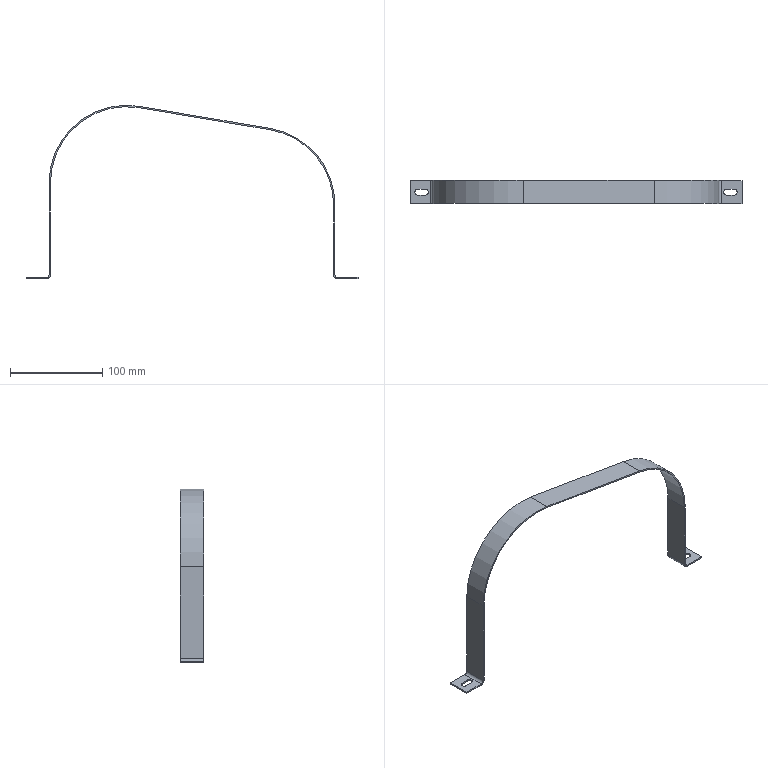Part | STEP file | 冲床-300配套压波_id546_x_t | 1 solid | 30 faces | box 360 x 25 x 188 mm | volume 23610 mm3 | plane 18 | cylinder 12 | commonest cylinder face diameters 6.5 x4 6 x2 9 x2 165 x2 168 x2
STEP:
#1=CARTESIAN_POINT('',(1167.5,-135.,104.));
#2=VERTEX_POINT('',#1);
#3=CARTESIAN_POINT('',(1167.5,-135.,4.5));
#4=VERTEX_POINT('',#3);
#5=CARTESIAN_POINT('',(1167.5,-135.,104.));
#6=DIRECTION('',(0.,0.,-1.));
#7=VECTOR('',#6,1.);
#8=LINE('',#5,#7);
#9=EDGE_CURVE('',#2,#4,#8,.T.);
#10=ORIENTED_EDGE('',*,*,#9,.F.);
#11=CARTESIAN_POINT('',(1263.702,-135.,185.354));
#12=VERTEX_POINT('',#11);
#13=CARTESIAN_POINT('',(1250.,-135.,104.));
#14=DIRECTION('',(0.,-1.,0.));
#15=DIRECTION('',(0.,0.,-1.));
#16=AXIS2_PLACEMENT_3D('',#13,#14,#15);
#17=CIRCLE('',#16,82.5);
#18=EDGE_CURVE('',#12,#2,#17,.T.);
#19=ORIENTED_EDGE('',*,*,#18,.F.);
#20=CARTESIAN_POINT('',(1405.702,-135.,161.438));
#21=VERTEX_POINT('',#20);
#22=CARTESIAN_POINT('',(1263.702,-135.,185.354));
#23=DIRECTION('',(-0.9861,0.,0.1661));
#24=VECTOR('',#23,1.);
#25=LINE('',#22,#24);
#26=EDGE_CURVE('',#21,#12,#25,.T.);
#27=ORIENTED_EDGE('',*,*,#26,.F.);
#28=CARTESIAN_POINT('',(1474.5,-135.,80.083));
#29=VERTEX_POINT('',#28);
#30=CARTESIAN_POINT('',(1392.,-135.,80.083));
#31=DIRECTION('',(0.,-1.,0.));
#32=DIRECTION('',(0.,0.,-1.));
#33=AXIS2_PLACEMENT_3D('',#30,#31,#32);
#34=CIRCLE('',#33,82.5);
#35=EDGE_CURVE('',#29,#21,#34,.T.);
#36=ORIENTED_EDGE('',*,*,#35,.F.);
#37=CARTESIAN_POINT('',(1474.5,-135.,4.5));
#38=VERTEX_POINT('',#37);
#39=CARTESIAN_POINT('',(1474.5,-135.,104.));
#40=DIRECTION('',(0.,0.,1.));
#41=VECTOR('',#40,1.);
#42=LINE('',#39,#41);
#43=EDGE_CURVE('',#38,#29,#42,.T.);
#44=ORIENTED_EDGE('',*,*,#43,.F.);
#45=CARTESIAN_POINT('',(1479.,-135.,0.));
#46=VERTEX_POINT('',#45);
#47=CARTESIAN_POINT('',(1479.,-135.,4.5));
#48=DIRECTION('',(0.,-1.,0.));
#49=DIRECTION('',(0.,0.,-1.));
#50=AXIS2_PLACEMENT_3D('',#47,#48,#49);
#51=CIRCLE('',#50,4.5);
#52=EDGE_CURVE('',#38,#46,#51,.T.);
#53=ORIENTED_EDGE('',*,*,#52,.T.);
#54=CARTESIAN_POINT('',(1501.,-135.,0.));
#55=VERTEX_POINT('',#54);
#56=CARTESIAN_POINT('',(1507.,-135.,0.));
#57=DIRECTION('',(1.,0.,0.));
#58=VECTOR('',#57,1.);
#59=LINE('',#56,#58);
#60=EDGE_CURVE('',#46,#55,#59,.T.);
#61=ORIENTED_EDGE('',*,*,#60,.T.);
#62=CARTESIAN_POINT('',(1501.,-135.,1.5));
#63=VERTEX_POINT('',#62);
#64=CARTESIAN_POINT('',(1501.,-135.,0.));
#65=DIRECTION('',(0.,0.,-1.));
#66=VECTOR('',#65,1.);
#67=LINE('',#64,#66);
#68=EDGE_CURVE('',#63,#55,#67,.T.);
#69=ORIENTED_EDGE('',*,*,#68,.F.);
#70=CARTESIAN_POINT('',(1479.,-135.,1.5));
#71=VERTEX_POINT('',#70);
#72=CARTESIAN_POINT('',(1507.,-135.,1.5));
#73=DIRECTION('',(1.,0.,0.));
#74=VECTOR('',#73,1.);
#75=LINE('',#72,#74);
#76=EDGE_CURVE('',#71,#63,#75,.T.);
#77=ORIENTED_EDGE('',*,*,#76,.F.);
#78=CARTESIAN_POINT('',(1476.,-135.,4.5));
#79=VERTEX_POINT('',#78);
#80=CARTESIAN_POINT('',(1479.,-135.,4.5));
#81=DIRECTION('',(0.,1.,0.));
#82=DIRECTION('',(0.,0.,-1.));
#83=AXIS2_PLACEMENT_3D('',#80,#81,#82);
#84=CIRCLE('',#83,3.);
#85=EDGE_CURVE('',#71,#79,#84,.T.);
#86=ORIENTED_EDGE('',*,*,#85,.T.);
#87=CARTESIAN_POINT('',(1476.,-135.,80.083));
#88=VERTEX_POINT('',#87);
#89=CARTESIAN_POINT('',(1476.,-135.,104.));
#90=DIRECTION('',(0.,0.,1.));
#91=VECTOR('',#90,1.);
#92=LINE('',#89,#91);
#93=EDGE_CURVE('',#79,#88,#92,.T.);
#94=ORIENTED_EDGE('',*,*,#93,.T.);
#95=CARTESIAN_POINT('',(1405.951,-135.,162.917));
#96=VERTEX_POINT('',#95);
#97=CARTESIAN_POINT('',(1392.,-135.,80.083));
#98=DIRECTION('',(0.,-1.,0.));
#99=DIRECTION('',(0.,0.,-1.));
#100=AXIS2_PLACEMENT_3D('',#97,#98,#99);
#101=CIRCLE('',#100,84.);
#102=EDGE_CURVE('',#88,#96,#101,.T.);
#103=ORIENTED_EDGE('',*,*,#102,.T.);
#104=CARTESIAN_POINT('',(1263.951,-135.,186.833));
#105=VERTEX_POINT('',#104);
#106=CARTESIAN_POINT('',(1263.951,-135.,186.833));
#107=DIRECTION('',(-0.9861,0.,0.1661));
#108=VECTOR('',#107,1.);
#109=LINE('',#106,#108);
#110=EDGE_CURVE('',#96,#105,#109,.T.);
#111=ORIENTED_EDGE('',*,*,#110,.T.);
#112=CARTESIAN_POINT('',(1166.,-135.,104.));
#113=VERTEX_POINT('',#112);
#114=CARTESIAN_POINT('',(1250.,-135.,104.));
#115=DIRECTION('',(0.,-1.,0.));
#116=DIRECTION('',(0.,0.,-1.));
#117=AXIS2_PLACEMENT_3D('',#114,#115,#116);
#118=CIRCLE('',#117,84.);
#119=EDGE_CURVE('',#105,#113,#118,.T.);
#120=ORIENTED_EDGE('',*,*,#119,.T.);
#121=CARTESIAN_POINT('',(1166.,-135.,4.5));
#122=VERTEX_POINT('',#121);
#123=CARTESIAN_POINT('',(1166.,-135.,104.));
#124=DIRECTION('',(0.,0.,1.));
#125=VECTOR('',#124,1.);
#126=LINE('',#123,#125);
#127=EDGE_CURVE('',#122,#113,#126,.T.);
#128=ORIENTED_EDGE('',*,*,#127,.F.);
#129=CARTESIAN_POINT('',(1163.,-135.,1.5));
#130=VERTEX_POINT('',#129);
#131=CARTESIAN_POINT('',(1163.,-135.,4.5));
#132=DIRECTION('',(0.,1.,0.));
#133=DIRECTION('',(0.,0.,-1.));
#134=AXIS2_PLACEMENT_3D('',#131,#132,#133);
#135=CIRCLE('',#134,3.);
#136=EDGE_CURVE('',#122,#130,#135,.T.);
#137=ORIENTED_EDGE('',*,*,#136,.T.);
#138=CARTESIAN_POINT('',(1141.,-135.,1.5));
#139=VERTEX_POINT('',#138);
#140=CARTESIAN_POINT('',(1165.,-135.,1.5));
#141=DIRECTION('',(1.,0.,0.));
#142=VECTOR('',#141,1.);
#143=LINE('',#140,#142);
#144=EDGE_CURVE('',#139,#130,#143,.T.);
#145=ORIENTED_EDGE('',*,*,#144,.F.);
#146=CARTESIAN_POINT('',(1141.,-135.,0.));
#147=VERTEX_POINT('',#146);
#148=CARTESIAN_POINT('',(1141.,-135.,-20.));
#149=DIRECTION('',(0.,0.,1.));
#150=VECTOR('',#149,1.);
#151=LINE('',#148,#150);
#152=EDGE_CURVE('',#147,#139,#151,.T.);
#153=ORIENTED_EDGE('',*,*,#152,.F.);
#154=CARTESIAN_POINT('',(1163.,-135.,0.));
#155=VERTEX_POINT('',#154);
#156=CARTESIAN_POINT('',(1507.,-135.,0.));
#157=DIRECTION('',(1.,0.,0.));
#158=VECTOR('',#157,1.);
#159=LINE('',#156,#158);
#160=EDGE_CURVE('',#147,#155,#159,.T.);
#161=ORIENTED_EDGE('',*,*,#160,.T.);
#162=CARTESIAN_POINT('',(1163.,-135.,4.5));
#163=DIRECTION('',(0.,-1.,0.));
#164=DIRECTION('',(0.,0.,-1.));
#165=AXIS2_PLACEMENT_3D('',#162,#163,#164);
#166=CIRCLE('',#165,4.5);
#167=EDGE_CURVE('',#155,#4,#166,.T.);
#168=ORIENTED_EDGE('',*,*,#167,.T.);
#169=EDGE_LOOP('',(#10,#19,#27,#36,#44,#53,#61,#69,#77,#86,#94,#103,#111,#120,#128,#137,#145,#153,#161,#168));
#170=FACE_OUTER_BOUND('',#169,.T.);
#171=CARTESIAN_POINT('',(1250.,-135.,104.));
#172=DIRECTION('',(0.,-1.,0.));
#173=DIRECTION('',(0.9861,0.,-0.1661));
#174=AXIS2_PLACEMENT_3D('',#171,#172,#173);
#175=PLANE('',#174);
#176=ADVANCED_FACE('',(#170),#175,.T.);
#177=CARTESIAN_POINT('',(1474.5,-110.,4.5));
#178=VERTEX_POINT('',#177);
#179=CARTESIAN_POINT('',(1474.5,-71.5,4.5));
#180=DIRECTION('',(0.,-1.,0.));
#181=VECTOR('',#180,1.);
#182=LINE('',#179,#181);
#183=EDGE_CURVE('',#178,#38,#182,.T.);
#184=ORIENTED_EDGE('',*,*,#183,.T.);
#185=ORIENTED_EDGE('',*,*,#43,.T.);
#186=CARTESIAN_POINT('',(1474.5,-110.,80.083));
#187=VERTEX_POINT('',#186);
#188=CARTESIAN_POINT('',(1474.5,-71.5,80.083));
#189=DIRECTION('',(0.,-1.,0.));
#190=VECTOR('',#189,1.);
#191=LINE('',#188,#190);
#192=EDGE_CURVE('',#187,#29,#191,.T.);
#193=ORIENTED_EDGE('',*,*,#192,.F.);
#194=CARTESIAN_POINT('',(1474.5,-110.,0.));
#195=DIRECTION('',(0.,0.,1.));
#196=VECTOR('',#195,1.);
#197=LINE('',#194,#196);
#198=EDGE_CURVE('',#178,#187,#197,.T.);
#199=ORIENTED_EDGE('',*,*,#198,.F.);
#200=EDGE_LOOP('',(#184,#185,#193,#199));
#201=FACE_OUTER_BOUND('',#200,.T.);
#202=CARTESIAN_POINT('',(1474.5,-71.5,0.));
#203=DIRECTION('',(1.,0.,0.));
#204=DIRECTION('',(0.,0.,-1.));
#205=AXIS2_PLACEMENT_3D('',#202,#203,#204);
#206=PLANE('',#205);
#207=ADVANCED_FACE('',(#201),#206,.F.);
#208=ORIENTED_EDGE('',*,*,#192,.T.);
#209=ORIENTED_EDGE('',*,*,#35,.T.);
#210=CARTESIAN_POINT('',(1405.702,-110.,161.438));
#211=VERTEX_POINT('',#210);
#212=CARTESIAN_POINT('',(1405.702,-71.5,161.438));
#213=DIRECTION('',(0.,-1.,0.));
#214=VECTOR('',#213,1.);
#215=LINE('',#212,#214);
#216=EDGE_CURVE('',#211,#21,#215,.T.);
#217=ORIENTED_EDGE('',*,*,#216,.F.);
#218=CARTESIAN_POINT('',(1392.,-110.,80.083));
#219=DIRECTION('',(0.,-1.,0.));
#220=DIRECTION('',(0.,0.,1.));
#221=AXIS2_PLACEMENT_3D('',#218,#219,#220);
#222=CIRCLE('',#221,82.5);
#223=EDGE_CURVE('',#187,#211,#222,.T.);
#224=ORIENTED_EDGE('',*,*,#223,.F.);
#225=EDGE_LOOP('',(#208,#209,#217,#224));
#226=FACE_OUTER_BOUND('',#225,.T.);
#227=CARTESIAN_POINT('',(1392.,-71.5,80.083));
#228=DIRECTION('',(0.,-1.,0.));
#229=DIRECTION('',(0.,0.,-1.));
#230=AXIS2_PLACEMENT_3D('',#227,#228,#229);
#231=CYLINDRICAL_SURFACE('',#230,82.5);
#232=ADVANCED_FACE('',(#226),#231,.F.);
#233=ORIENTED_EDGE('',*,*,#144,.T.);
#234=CARTESIAN_POINT('',(1163.,-110.,1.5));
#235=VERTEX_POINT('',#234);
#236=CARTESIAN_POINT('',(1163.,-110.,1.5));
#237=DIRECTION('',(0.,1.,0.));
#238=VECTOR('',#237,1.);
#239=LINE('',#236,#238);
#240=EDGE_CURVE('',#130,#235,#239,.T.);
#241=ORIENTED_EDGE('',*,*,#240,.T.);
#242=CARTESIAN_POINT('',(1141.,-110.,1.5));
#243=VERTEX_POINT('',#242);
#244=CARTESIAN_POINT('',(1165.,-110.,1.5));
#245=DIRECTION('',(-1.,0.,0.));
#246=VECTOR('',#245,1.);
#247=LINE('',#244,#246);
#248=EDGE_CURVE('',#235,#243,#247,.T.);
#249=ORIENTED_EDGE('',*,*,#248,.T.);
#250=CARTESIAN_POINT('',(1141.,-71.5,1.5));
#251=DIRECTION('',(0.,-1.,0.));
#252=VECTOR('',#251,1.);
#253=LINE('',#250,#252);
#254=EDGE_CURVE('',#243,#139,#253,.T.);
#255=ORIENTED_EDGE('',*,*,#254,.T.);
#256=EDGE_LOOP('',(#233,#241,#249,#255));
#257=FACE_BOUND('',#256,.T.);
#258=CARTESIAN_POINT('',(1157.5,-125.75,1.5));
#259=VERTEX_POINT('',#258);
#260=CARTESIAN_POINT('',(1149.5,-125.75,1.5));
#261=VERTEX_POINT('',#260);
#262=CARTESIAN_POINT('',(1163.5,-125.75,1.5));
#263=DIRECTION('',(-1.,0.,0.));
#264=VECTOR('',#263,1.);
#265=LINE('',#262,#264);
#266=EDGE_CURVE('',#259,#261,#265,.T.);
#267=ORIENTED_EDGE('',*,*,#266,.T.);
#268=CARTESIAN_POINT('',(1149.5,-119.25,1.5));
#269=VERTEX_POINT('',#268);
#270=CARTESIAN_POINT('',(1149.5,-122.5,1.5));
#271=DIRECTION('',(0.,0.,-1.));
#272=DIRECTION('',(1.,0.,0.));
#273=AXIS2_PLACEMENT_3D('',#270,#271,#272);
#274=CIRCLE('',#273,3.25);
#275=EDGE_CURVE('',#261,#269,#274,.T.);
#276=ORIENTED_EDGE('',*,*,#275,.T.);
#277=CARTESIAN_POINT('',(1157.5,-119.25,1.5));
#278=VERTEX_POINT('',#277);
#279=CARTESIAN_POINT('',(1163.5,-119.25,1.5));
#280=DIRECTION('',(1.,0.,0.));
#281=VECTOR('',#280,1.);
#282=LINE('',#279,#281);
#283=EDGE_CURVE('',#269,#278,#282,.T.);
#284=ORIENTED_EDGE('',*,*,#283,.T.);
#285=CARTESIAN_POINT('',(1157.5,-122.5,1.5));
#286=DIRECTION('',(0.,0.,-1.));
#287=DIRECTION('',(1.,0.,0.));
#288=AXIS2_PLACEMENT_3D('',#285,#286,#287);
#289=CIRCLE('',#288,3.25);
#290=EDGE_CURVE('',#278,#259,#289,.T.);
#291=ORIENTED_EDGE('',*,*,#290,.T.);
#292=EDGE_LOOP('',(#267,#276,#284,#291));
#293=FACE_BOUND('',#292,.T.);
#294=CARTESIAN_POINT('',(1165.,-71.5,1.5));
#295=DIRECTION('',(0.,0.,1.));
#296=DIRECTION('',(1.,0.,0.));
#297=AXIS2_PLACEMENT_3D('',#294,#295,#296);
#298=PLANE('',#297);
#299=ADVANCED_FACE('',(#257,#293),#298,.T.);
#300=CARTESIAN_POINT('',(1163.,-110.,0.));
#301=VERTEX_POINT('',#300);
#302=CARTESIAN_POINT('',(1141.,-110.,0.));
#303=VERTEX_POINT('',#302);
#304=CARTESIAN_POINT('',(1507.,-110.,0.));
#305=DIRECTION('',(-1.,0.,0.));
#306=VECTOR('',#305,1.);
#307=LINE('',#304,#306);
#308=EDGE_CURVE('',#301,#303,#307,.T.);
#309=ORIENTED_EDGE('',*,*,#308,.F.);
#310=CARTESIAN_POINT('',(1163.,-71.5,0.));
#311=DIRECTION('',(0.,-1.,0.));
#312=VECTOR('',#311,1.);
#313=LINE('',#310,#312);
#314=EDGE_CURVE('',#301,#155,#313,.T.);
#315=ORIENTED_EDGE('',*,*,#314,.T.);
#316=ORIENTED_EDGE('',*,*,#160,.F.);
#317=CARTESIAN_POINT('',(1141.,-71.5,0.));
#318=DIRECTION('',(0.,-1.,0.));
#319=VECTOR('',#318,1.);
#320=LINE('',#317,#319);
#321=EDGE_CURVE('',#303,#147,#320,.T.);
#322=ORIENTED_EDGE('',*,*,#321,.F.);
#323=EDGE_LOOP('',(#309,#315,#316,#322));
#324=FACE_BOUND('',#323,.T.);
#325=CARTESIAN_POINT('',(1149.5,-125.75,0.));
#326=VERTEX_POINT('',#325);
#327=CARTESIAN_POINT('',(1149.5,-119.25,0.));
#328=VERTEX_POINT('',#327);
#329=CARTESIAN_POINT('',(1149.5,-122.5,0.));
#330=DIRECTION('',(0.,0.,-1.));
#331=DIRECTION('',(1.,0.,0.));
#332=AXIS2_PLACEMENT_3D('',#329,#330,#331);
#333=CIRCLE('',#332,3.25);
#334=EDGE_CURVE('',#326,#328,#333,.T.);
#335=ORIENTED_EDGE('',*,*,#334,.F.);
#336=CARTESIAN_POINT('',(1157.5,-125.75,0.));
#337=VERTEX_POINT('',#336);
#338=CARTESIAN_POINT('',(1505.5,-125.75,0.));
#339=DIRECTION('',(-1.,0.,0.));
#340=VECTOR('',#339,1.);
#341=LINE('',#338,#340);
#342=EDGE_CURVE('',#337,#326,#341,.T.);
#343=ORIENTED_EDGE('',*,*,#342,.F.);
#344=CARTESIAN_POINT('',(1157.5,-119.25,0.));
#345=VERTEX_POINT('',#344);
#346=CARTESIAN_POINT('',(1157.5,-122.5,0.));
#347=DIRECTION('',(0.,0.,-1.));
#348=DIRECTION('',(1.,0.,0.));
#349=AXIS2_PLACEMENT_3D('',#346,#347,#348);
#350=CIRCLE('',#349,3.25);
#351=EDGE_CURVE('',#345,#337,#350,.T.);
#352=ORIENTED_EDGE('',*,*,#351,.F.);
#353=CARTESIAN_POINT('',(1505.5,-119.25,0.));
#354=DIRECTION('',(1.,0.,0.));
#355=VECTOR('',#354,1.);
#356=LINE('',#353,#355);
#357=EDGE_CURVE('',#328,#345,#356,.T.);
#358=ORIENTED_EDGE('',*,*,#357,.F.);
#359=EDGE_LOOP('',(#335,#343,#352,#358));
#360=FACE_BOUND('',#359,.T.);
#361=CARTESIAN_POINT('',(1507.,-71.5,0.));
#362=DIRECTION('',(0.,0.,1.));
#363=DIRECTION('',(1.,0.,0.));
#364=AXIS2_PLACEMENT_3D('',#361,#362,#363);
#365=PLANE('',#364);
#366=ADVANCED_FACE('',(#324,#360),#365,.F.);
#367=CARTESIAN_POINT('',(1492.5,-125.75,0.));
#368=VERTEX_POINT('',#367);
#369=CARTESIAN_POINT('',(1484.5,-125.75,0.));
#370=VERTEX_POINT('',#369);
#371=CARTESIAN_POINT('',(1509.5,-125.75,0.));
#372=DIRECTION('',(-1.,0.,0.));
#373=VECTOR('',#372,1.);
#374=LINE('',#371,#373);
#375=EDGE_CURVE('',#368,#370,#374,.T.);
#376=ORIENTED_EDGE('',*,*,#375,.F.);
#377=CARTESIAN_POINT('',(1492.5,-119.25,0.));
#378=VERTEX_POINT('',#377);
#379=CARTESIAN_POINT('',(1492.5,-122.5,0.));
#380=DIRECTION('',(0.,0.,-1.));
#381=DIRECTION('',(1.,0.,0.));
#382=AXIS2_PLACEMENT_3D('',#379,#380,#381);
#383=CIRCLE('',#382,3.25);
#384=EDGE_CURVE('',#378,#368,#383,.T.);
#385=ORIENTED_EDGE('',*,*,#384,.F.);
#386=CARTESIAN_POINT('',(1484.5,-119.25,0.));
#387=VERTEX_POINT('',#386);
#388=CARTESIAN_POINT('',(1509.5,-119.25,0.));
#389=DIRECTION('',(1.,0.,0.));
#390=VECTOR('',#389,1.);
#391=LINE('',#388,#390);
#392=EDGE_CURVE('',#387,#378,#391,.T.);
#393=ORIENTED_EDGE('',*,*,#392,.F.);
#394=CARTESIAN_POINT('',(1484.5,-122.5,0.));
#395=DIRECTION('',(0.,0.,-1.));
#396=DIRECTION('',(1.,0.,0.));
#397=AXIS2_PLACEMENT_3D('',#394,#395,#396);
#398=CIRCLE('',#397,3.25);
#399=EDGE_CURVE('',#370,#387,#398,.T.);
#400=ORIENTED_EDGE('',*,*,#399,.F.);
#401=EDGE_LOOP('',(#376,#385,#393,#400));
#402=FACE_BOUND('',#401,.T.);
#403=ORIENTED_EDGE('',*,*,#60,.F.);
#404=CARTESIAN_POINT('',(1479.,-110.,0.));
#405=VERTEX_POINT('',#404);
#406=CARTESIAN_POINT('',(1479.,-71.5,0.));
#407=DIRECTION('',(0.,1.,0.));
#408=VECTOR('',#407,1.);
#409=LINE('',#406,#408);
#410=EDGE_CURVE('',#46,#405,#409,.T.);
#411=ORIENTED_EDGE('',*,*,#410,.T.);
#412=CARTESIAN_POINT('',(1501.,-110.,0.));
#413=VERTEX_POINT('',#412);
#414=CARTESIAN_POINT('',(1507.,-110.,0.));
#415=DIRECTION('',(-1.,0.,0.));
#416=VECTOR('',#415,1.);
#417=LINE('',#414,#416);
#418=EDGE_CURVE('',#413,#405,#417,.T.);
#419=ORIENTED_EDGE('',*,*,#418,.F.);
#420=CARTESIAN_POINT('',(1501.,-71.5,0.));
#421=DIRECTION('',(0.,-1.,0.));
#422=VECTOR('',#421,1.);
#423=LINE('',#420,#422);
#424=EDGE_CURVE('',#413,#55,#423,.T.);
#425=ORIENTED_EDGE('',*,*,#424,.T.);
#426=EDGE_LOOP('',(#403,#411,#419,#425));
#427=FACE_BOUND('',#426,.T.);
#428=CARTESIAN_POINT('',(1507.,-71.5,0.));
#429=DIRECTION('',(0.,0.,1.));
#430=DIRECTION('',(1.,0.,0.));
#431=AXIS2_PLACEMENT_3D('',#428,#429,#430);
#432=PLANE('',#431);
#433=ADVANCED_FACE('',(#402,#427),#432,.F.);
#434=CARTESIAN_POINT('',(1476.,-110.,80.083));
#435=VERTEX_POINT('',#434);
#436=CARTESIAN_POINT('',(1476.,-71.5,80.083));
#437=DIRECTION('',(0.,1.,0.));
#438=VECTOR('',#437,1.);
#439=LINE('',#436,#438);
#440=EDGE_CURVE('',#88,#435,#439,.T.);
#441=ORIENTED_EDGE('',*,*,#440,.T.);
#442=CARTESIAN_POINT('',(1405.951,-110.,162.917));
#443=VERTEX_POINT('',#442);
#444=CARTESIAN_POINT('',(1392.,-110.,80.083));
#445=DIRECTION('',(0.,-1.,0.));
#446=DIRECTION('',(0.,0.,1.));
#447=AXIS2_PLACEMENT_3D('',#444,#445,#446);
#448=CIRCLE('',#447,84.);
#449=EDGE_CURVE('',#435,#443,#448,.T.);
#450=ORIENTED_EDGE('',*,*,#449,.T.);
#451=CARTESIAN_POINT('',(1405.951,-71.5,162.917));
#452=DIRECTION('',(0.,1.,0.));
#453=VECTOR('',#452,1.);
#454=LINE('',#451,#453);
#455=EDGE_CURVE('',#96,#443,#454,.T.);
#456=ORIENTED_EDGE('',*,*,#455,.F.);
#457=ORIENTED_EDGE('',*,*,#102,.F.);
#458=EDGE_LOOP('',(#441,#450,#456,#457));
#459=FACE_OUTER_BOUND('',#458,.T.);
#460=CARTESIAN_POINT('',(1392.,-71.5,80.083));
#461=DIRECTION('',(0.,-1.,0.));
#462=DIRECTION('',(0.,0.,-1.));
#463=AXIS2_PLACEMENT_3D('',#460,#461,#462);
#464=CYLINDRICAL_SURFACE('',#463,84.);
#465=ADVANCED_FACE('',(#459),#464,.T.);
#466=CARTESIAN_POINT('',(1263.951,-110.,186.833));
#467=VERTEX_POINT('',#466);
#468=CARTESIAN_POINT('',(1263.951,-71.5,186.833));
#469=DIRECTION('',(0.,1.,0.));
#470=VECTOR('',#469,1.);
#471=LINE('',#468,#470);
#472=EDGE_CURVE('',#105,#467,#471,.T.);
#473=ORIENTED_EDGE('',*,*,#472,.T.);
#474=CARTESIAN_POINT('',(1166.,-110.,104.));
#475=VERTEX_POINT('',#474);
#476=CARTESIAN_POINT('',(1250.,-110.,104.));
#477=DIRECTION('',(0.,-1.,0.));
#478=DIRECTION('',(0.,0.,1.));
#479=AXIS2_PLACEMENT_3D('',#476,#477,#478);
#480=CIRCLE('',#479,84.);
#481=EDGE_CURVE('',#467,#475,#480,.T.);
#482=ORIENTED_EDGE('',*,*,#481,.T.);
#483=CARTESIAN_POINT('',(1166.,-71.5,104.));
#484=DIRECTION('',(0.,1.,0.));
#485=VECTOR('',#484,1.);
#486=LINE('',#483,#485);
#487=EDGE_CURVE('',#113,#475,#486,.T.);
#488=ORIENTED_EDGE('',*,*,#487,.F.);
#489=ORIENTED_EDGE('',*,*,#119,.F.);
#490=EDGE_LOOP('',(#473,#482,#488,#489));
#491=FACE_OUTER_BOUND('',#490,.T.);
#492=CARTESIAN_POINT('',(1250.,-71.5,104.));
#493=DIRECTION('',(0.,-1.,0.));
#494=DIRECTION('',(0.,0.,-1.));
#495=AXIS2_PLACEMENT_3D('',#492,#493,#494);
#496=CYLINDRICAL_SURFACE('',#495,84.);
#497=ADVANCED_FACE('',(#491),#496,.T.);
#498=ORIENTED_EDGE('',*,*,#254,.F.);
#499=CARTESIAN_POINT('',(1141.,-110.,-20.));
#500=DIRECTION('',(0.,0.,-1.));
#501=VECTOR('',#500,1.);
#502=LINE('',#499,#501);
#503=EDGE_CURVE('',#243,#303,#502,.T.);
#504=ORIENTED_EDGE('',*,*,#503,.T.);
#505=ORIENTED_EDGE('',*,*,#321,.T.);
#506=ORIENTED_EDGE('',*,*,#152,.T.);
#507=EDGE_LOOP('',(#498,#504,#505,#506));
#508=FACE_OUTER_BOUND('',#507,.T.);
#509=CARTESIAN_POINT('',(1141.,300.,-20.));
#510=DIRECTION('',(-1.,0.,0.));
#511=DIRECTION('',(0.,0.,1.));
#512=AXIS2_PLACEMENT_3D('',#509,#510,#511);
#513=PLANE('',#512);
#514=ADVANCED_FACE('',(#508),#513,.T.);
#515=ORIENTED_EDGE('',*,*,#424,.F.);
#516=CARTESIAN_POINT('',(1501.,-110.,1.5));
#517=VERTEX_POINT('',#516);
#518=CARTESIAN_POINT('',(1501.,-110.,0.));
#519=DIRECTION('',(0.,0.,1.));
#520=VECTOR('',#519,1.);
#521=LINE('',#518,#520);
#522=EDGE_CURVE('',#413,#517,#521,.T.);
#523=ORIENTED_EDGE('',*,*,#522,.T.);
#524=CARTESIAN_POINT('',(1501.,-71.5,1.5));
#525=DIRECTION('',(0.,-1.,0.));
#526=VECTOR('',#525,1.);
#527=LINE('',#524,#526);
#528=EDGE_CURVE('',#517,#63,#527,.T.);
#529=ORIENTED_EDGE('',*,*,#528,.T.);
#530=ORIENTED_EDGE('',*,*,#68,.T.);
#531=EDGE_LOOP('',(#515,#523,#529,#530));
#532=FACE_OUTER_BOUND('',#531,.T.);
#533=CARTESIAN_POINT('',(1501.,-71.5,0.));
#534=DIRECTION('',(-1.,0.,0.));
#535=DIRECTION('',(0.,-1.,0.));
#536=AXIS2_PLACEMENT_3D('',#533,#534,#535);
#537=PLANE('',#536);
#538=ADVANCED_FACE('',(#532),#537,.F.);
#539=CARTESIAN_POINT('',(1492.5,-119.25,1.5));
#540=VERTEX_POINT('',#539);
#541=CARTESIAN_POINT('',(1492.5,-125.75,1.5));
#542=VERTEX_POINT('',#541);
#543=CARTESIAN_POINT('',(1492.5,-122.5,1.5));
#544=DIRECTION('',(0.,0.,-1.));
#545=DIRECTION('',(1.,0.,0.));
#546=AXIS2_PLACEMENT_3D('',#543,#544,#545);
#547=CIRCLE('',#546,3.25);
#548=EDGE_CURVE('',#540,#542,#547,.T.);
#549=ORIENTED_EDGE('',*,*,#548,.T.);
#550=CARTESIAN_POINT('',(1484.5,-125.75,1.5));
#551=VERTEX_POINT('',#550);
#552=CARTESIAN_POINT('',(1509.5,-125.75,1.5));
#553=DIRECTION('',(-1.,0.,0.));
#554=VECTOR('',#553,1.);
#555=LINE('',#552,#554);
#556=EDGE_CURVE('',#542,#551,#555,.T.);
#557=ORIENTED_EDGE('',*,*,#556,.T.);
#558=CARTESIAN_POINT('',(1484.5,-119.25,1.5));
#559=VERTEX_POINT('',#558);
#560=CARTESIAN_POINT('',(1484.5,-122.5,1.5));
#561=DIRECTION('',(0.,0.,-1.));
#562=DIRECTION('',(1.,0.,0.));
#563=AXIS2_PLACEMENT_3D('',#560,#561,#562);
#564=CIRCLE('',#563,3.25);
#565=EDGE_CURVE('',#551,#559,#564,.T.);
#566=ORIENTED_EDGE('',*,*,#565,.T.);
#567=CARTESIAN_POINT('',(1509.5,-119.25,1.5));
#568=DIRECTION('',(1.,0.,0.));
#569=VECTOR('',#568,1.);
#570=LINE('',#567,#569);
#571=EDGE_CURVE('',#559,#540,#570,.T.);
#572=ORIENTED_EDGE('',*,*,#571,.T.);
#573=EDGE_LOOP('',(#549,#557,#566,#572));
#574=FACE_BOUND('',#573,.T.);
#575=CARTESIAN_POINT('',(1479.,-110.,1.5));
#576=VERTEX_POINT('',#575);
#577=CARTESIAN_POINT('',(1507.,-110.,1.5));
#578=DIRECTION('',(-1.,0.,0.));
#579=VECTOR('',#578,1.);
#580=LINE('',#577,#579);
#581=EDGE_CURVE('',#517,#576,#580,.T.);
#582=ORIENTED_EDGE('',*,*,#581,.T.);
#583=CARTESIAN_POINT('',(1479.,-135.,1.5));
#584=DIRECTION('',(0.,-1.,0.));
#585=VECTOR('',#584,1.);
#586=LINE('',#583,#585);
#587=EDGE_CURVE('',#576,#71,#586,.T.);
#588=ORIENTED_EDGE('',*,*,#587,.T.);
#589=ORIENTED_EDGE('',*,*,#76,.T.);
#590=ORIENTED_EDGE('',*,*,#528,.F.);
#591=EDGE_LOOP('',(#582,#588,#589,#590));
#592=FACE_BOUND('',#591,.T.);
#593=CARTESIAN_POINT('',(1507.,-71.5,1.5));
#594=DIRECTION('',(0.,0.,1.));
#595=DIRECTION('',(1.,0.,0.));
#596=AXIS2_PLACEMENT_3D('',#593,#594,#595);
#597=PLANE('',#596);
#598=ADVANCED_FACE('',(#574,#592),#597,.T.);
#599=ORIENTED_EDGE('',*,*,#93,.F.);
#600=CARTESIAN_POINT('',(1476.,-110.,4.5));
#601=VERTEX_POINT('',#600);
#602=CARTESIAN_POINT('',(1476.,-110.,4.5));
#603=DIRECTION('',(0.,1.,0.));
#604=VECTOR('',#603,1.);
#605=LINE('',#602,#604);
#606=EDGE_CURVE('',#79,#601,#605,.T.);
#607=ORIENTED_EDGE('',*,*,#606,.T.);
#608=CARTESIAN_POINT('',(1476.,-110.,0.));
#609=DIRECTION('',(0.,0.,1.));
#610=VECTOR('',#609,1.);
#611=LINE('',#608,#610);
#612=EDGE_CURVE('',#601,#435,#611,.T.);
#613=ORIENTED_EDGE('',*,*,#612,.T.);
#614=ORIENTED_EDGE('',*,*,#440,.F.);
#615=EDGE_LOOP('',(#599,#607,#613,#614));
#616=FACE_OUTER_BOUND('',#615,.T.);
#617=CARTESIAN_POINT('',(1476.,-71.5,0.));
#618=DIRECTION('',(1.,0.,0.));
#619=DIRECTION('',(0.,0.,-1.));
#620=AXIS2_PLACEMENT_3D('',#617,#618,#619);
#621=PLANE('',#620);
#622=ADVANCED_FACE('',(#616),#621,.T.);
#623=ORIENTED_EDGE('',*,*,#455,.T.);
#624=CARTESIAN_POINT('',(1405.951,-110.,162.917));
#625=DIRECTION('',(-0.9861,0.,0.1661));
#626=VECTOR('',#625,1.);
#627=LINE('',#624,#626);
#628=EDGE_CURVE('',#443,#467,#627,.T.);
#629=ORIENTED_EDGE('',*,*,#628,.T.);
#630=ORIENTED_EDGE('',*,*,#472,.F.);
#631=ORIENTED_EDGE('',*,*,#110,.F.);
#632=EDGE_LOOP('',(#623,#629,#630,#631));
#633=FACE_OUTER_BOUND('',#632,.T.);
#634=CARTESIAN_POINT('',(1405.951,-71.5,162.917));
#635=DIRECTION('',(0.1661,0.,0.9861));
#636=DIRECTION('',(0.9861,0.,-0.1661));
#637=AXIS2_PLACEMENT_3D('',#634,#635,#636);
#638=PLANE('',#637);
#639=ADVANCED_FACE('',(#633),#638,.T.);
#640=CARTESIAN_POINT('',(1166.,-110.,4.5));
#641=VERTEX_POINT('',#640);
#642=CARTESIAN_POINT('',(1166.,-110.,104.));
#643=DIRECTION('',(0.,0.,-1.));
#644=VECTOR('',#643,1.);
#645=LINE('',#642,#644);
#646=EDGE_CURVE('',#475,#641,#645,.T.);
#647=ORIENTED_EDGE('',*,*,#646,.T.);
#648=CARTESIAN_POINT('',(1166.,-135.,4.5));
#649=DIRECTION('',(0.,-1.,0.));
#650=VECTOR('',#649,1.);
#651=LINE('',#648,#650);
#652=EDGE_CURVE('',#641,#122,#651,.T.);
#653=ORIENTED_EDGE('',*,*,#652,.T.);
#654=ORIENTED_EDGE('',*,*,#127,.T.);
#655=ORIENTED_EDGE('',*,*,#487,.T.);
#656=EDGE_LOOP('',(#647,#653,#654,#655));
#657=FACE_OUTER_BOUND('',#656,.T.);
#658=CARTESIAN_POINT('',(1166.,-71.5,104.));
#659=DIRECTION('',(-1.,0.,0.));
#660=DIRECTION('',(0.,0.,1.));
#661=AXIS2_PLACEMENT_3D('',#658,#659,#660);
#662=PLANE('',#661);
#663=ADVANCED_FACE('',(#657),#662,.T.);
#664=CARTESIAN_POINT('',(1167.5,-110.,104.));
#665=VERTEX_POINT('',#664);
#666=CARTESIAN_POINT('',(1167.5,-110.,4.5));
#667=VERTEX_POINT('',#666);
#668=CARTESIAN_POINT('',(1167.5,-110.,104.));
#669=DIRECTION('',(0.,0.,-1.));
#670=VECTOR('',#669,1.);
#671=LINE('',#668,#670);
#672=EDGE_CURVE('',#665,#667,#671,.T.);
#673=ORIENTED_EDGE('',*,*,#672,.T.);
#674=CARTESIAN_POINT('',(1163.,-110.,4.5));
#675=DIRECTION('',(0.,1.,0.));
#676=DIRECTION('',(0.,0.,1.));
#677=AXIS2_PLACEMENT_3D('',#674,#675,#676);
#678=CIRCLE('',#677,4.5);
#679=EDGE_CURVE('',#667,#301,#678,.T.);
#680=ORIENTED_EDGE('',*,*,#679,.T.);
#681=ORIENTED_EDGE('',*,*,#308,.T.);
#682=ORIENTED_EDGE('',*,*,#503,.F.);
#683=ORIENTED_EDGE('',*,*,#248,.F.);
#684=CARTESIAN_POINT('',(1163.,-110.,4.5));
#685=DIRECTION('',(0.,-1.,0.));
#686=DIRECTION('',(0.,0.,1.));
#687=AXIS2_PLACEMENT_3D('',#684,#685,#686);
#688=CIRCLE('',#687,3.);
#689=EDGE_CURVE('',#235,#641,#688,.T.);
#690=ORIENTED_EDGE('',*,*,#689,.T.);
#691=ORIENTED_EDGE('',*,*,#646,.F.);
#692=ORIENTED_EDGE('',*,*,#481,.F.);
#693=ORIENTED_EDGE('',*,*,#628,.F.);
#694=ORIENTED_EDGE('',*,*,#449,.F.);
#695=ORIENTED_EDGE('',*,*,#612,.F.);
#696=CARTESIAN_POINT('',(1479.,-110.,4.5));
#697=DIRECTION('',(0.,-1.,0.));
#698=DIRECTION('',(0.,0.,1.));
#699=AXIS2_PLACEMENT_3D('',#696,#697,#698);
#700=CIRCLE('',#699,3.);
#701=EDGE_CURVE('',#601,#576,#700,.T.);
#702=ORIENTED_EDGE('',*,*,#701,.T.);
#703=ORIENTED_EDGE('',*,*,#581,.F.);
#704=ORIENTED_EDGE('',*,*,#522,.F.);
#705=ORIENTED_EDGE('',*,*,#418,.T.);
#706=CARTESIAN_POINT('',(1479.,-110.,4.5));
#707=DIRECTION('',(0.,1.,0.));
#708=DIRECTION('',(0.,0.,1.));
#709=AXIS2_PLACEMENT_3D('',#706,#707,#708);
#710=CIRCLE('',#709,4.5);
#711=EDGE_CURVE('',#405,#178,#710,.T.);
#712=ORIENTED_EDGE('',*,*,#711,.T.);
#713=ORIENTED_EDGE('',*,*,#198,.T.);
#714=ORIENTED_EDGE('',*,*,#223,.T.);
#715=CARTESIAN_POINT('',(1263.702,-110.,185.354));
#716=VERTEX_POINT('',#715);
#717=CARTESIAN_POINT('',(1405.702,-110.,161.438));
#718=DIRECTION('',(-0.9861,0.,0.1661));
#719=VECTOR('',#718,1.);
#720=LINE('',#717,#719);
#721=EDGE_CURVE('',#211,#716,#720,.T.);
#722=ORIENTED_EDGE('',*,*,#721,.T.);
#723=CARTESIAN_POINT('',(1250.,-110.,104.));
#724=DIRECTION('',(0.,-1.,0.));
#725=DIRECTION('',(0.,0.,1.));
#726=AXIS2_PLACEMENT_3D('',#723,#724,#725);
#727=CIRCLE('',#726,82.5);
#728=EDGE_CURVE('',#716,#665,#727,.T.);
#729=ORIENTED_EDGE('',*,*,#728,.T.);
#730=EDGE_LOOP('',(#673,#680,#681,#682,#683,#690,#691,#692,#693,#694,#695,#702,#703,#704,#705,#712,#713,#714,#722,#729));
#731=FACE_OUTER_BOUND('',#730,.T.);
#732=CARTESIAN_POINT('',(1250.,-110.,104.));
#733=DIRECTION('',(0.,1.,0.));
#734=DIRECTION('',(-0.9861,0.,0.1661));
#735=AXIS2_PLACEMENT_3D('',#732,#733,#734);
#736=PLANE('',#735);
#737=ADVANCED_FACE('',(#731),#736,.T.);
#738=CARTESIAN_POINT('',(1167.5,-71.5,104.));
#739=DIRECTION('',(0.,-1.,0.));
#740=VECTOR('',#739,1.);
#741=LINE('',#738,#740);
#742=EDGE_CURVE('',#665,#2,#741,.T.);
#743=ORIENTED_EDGE('',*,*,#742,.T.);
#744=ORIENTED_EDGE('',*,*,#9,.T.);
#745=CARTESIAN_POINT('',(1167.5,-71.5,4.5));
#746=DIRECTION('',(0.,1.,0.));
#747=VECTOR('',#746,1.);
#748=LINE('',#745,#747);
#749=EDGE_CURVE('',#4,#667,#748,.T.);
#750=ORIENTED_EDGE('',*,*,#749,.T.);
#751=ORIENTED_EDGE('',*,*,#672,.F.);
#752=EDGE_LOOP('',(#743,#744,#750,#751));
#753=FACE_OUTER_BOUND('',#752,.T.);
#754=CARTESIAN_POINT('',(1167.5,-71.5,104.));
#755=DIRECTION('',(-1.,0.,0.));
#756=DIRECTION('',(0.,0.,1.));
#757=AXIS2_PLACEMENT_3D('',#754,#755,#756);
#758=PLANE('',#757);
#759=ADVANCED_FACE('',(#753),#758,.F.);
#760=CARTESIAN_POINT('',(1263.702,-71.5,185.354));
#761=DIRECTION('',(0.,-1.,0.));
#762=VECTOR('',#761,1.);
#763=LINE('',#760,#762);
#764=EDGE_CURVE('',#716,#12,#763,.T.);
#765=ORIENTED_EDGE('',*,*,#764,.T.);
#766=ORIENTED_EDGE('',*,*,#18,.T.);
#767=ORIENTED_EDGE('',*,*,#742,.F.);
#768=ORIENTED_EDGE('',*,*,#728,.F.);
#769=EDGE_LOOP('',(#765,#766,#767,#768));
#770=FACE_OUTER_BOUND('',#769,.T.);
#771=CARTESIAN_POINT('',(1250.,-71.5,104.));
#772=DIRECTION('',(0.,-1.,0.));
#773=DIRECTION('',(0.,0.,-1.));
#774=AXIS2_PLACEMENT_3D('',#771,#772,#773);
#775=CYLINDRICAL_SURFACE('',#774,82.5);
#776=ADVANCED_FACE('',(#770),#775,.F.);
#777=ORIENTED_EDGE('',*,*,#216,.T.);
#778=ORIENTED_EDGE('',*,*,#26,.T.);
#779=ORIENTED_EDGE('',*,*,#764,.F.);
#780=ORIENTED_EDGE('',*,*,#721,.F.);
#781=EDGE_LOOP('',(#777,#778,#779,#780));
#782=FACE_OUTER_BOUND('',#781,.T.);
#783=CARTESIAN_POINT('',(1405.702,-71.5,161.438));
#784=DIRECTION('',(0.1661,0.,0.9861));
#785=DIRECTION('',(0.9861,0.,-0.1661));
#786=AXIS2_PLACEMENT_3D('',#783,#784,#785);
#787=PLANE('',#786);
#788=ADVANCED_FACE('',(#782),#787,.F.);
#789=CARTESIAN_POINT('',(1149.5,-125.75,-118.5));
#790=DIRECTION('',(0.,0.,-1.));
#791=VECTOR('',#790,1.);
#792=LINE('',#789,#791);
#793=EDGE_CURVE('',#261,#326,#792,.T.);
#794=ORIENTED_EDGE('',*,*,#793,.T.);
#795=ORIENTED_EDGE('',*,*,#334,.T.);
#796=CARTESIAN_POINT('',(1149.5,-119.25,-118.5));
#797=DIRECTION('',(0.,0.,-1.));
#798=VECTOR('',#797,1.);
#799=LINE('',#796,#798);
#800=EDGE_CURVE('',#269,#328,#799,.T.);
#801=ORIENTED_EDGE('',*,*,#800,.F.);
#802=ORIENTED_EDGE('',*,*,#275,.F.);
#803=EDGE_LOOP('',(#794,#795,#801,#802));
#804=FACE_OUTER_BOUND('',#803,.T.);
#805=CARTESIAN_POINT('',(1149.5,-122.5,-118.5));
#806=DIRECTION('',(0.,0.,1.));
#807=DIRECTION('',(1.,0.,0.));
#808=AXIS2_PLACEMENT_3D('',#805,#806,#807);
#809=CYLINDRICAL_SURFACE('',#808,3.25);
#810=ADVANCED_FACE('',(#804),#809,.F.);
#811=ORIENTED_EDGE('',*,*,#800,.T.);
#812=ORIENTED_EDGE('',*,*,#357,.T.);
#813=CARTESIAN_POINT('',(1157.5,-119.25,-118.5));
#814=DIRECTION('',(0.,0.,-1.));
#815=VECTOR('',#814,1.);
#816=LINE('',#813,#815);
#817=EDGE_CURVE('',#278,#345,#816,.T.);
#818=ORIENTED_EDGE('',*,*,#817,.F.);
#819=ORIENTED_EDGE('',*,*,#283,.F.);
#820=EDGE_LOOP('',(#811,#812,#818,#819));
#821=FACE_OUTER_BOUND('',#820,.T.);
#822=CARTESIAN_POINT('',(1149.5,-119.25,-118.5));
#823=DIRECTION('',(0.,-1.,0.));
#824=DIRECTION('',(0.,0.,-1.));
#825=AXIS2_PLACEMENT_3D('',#822,#823,#824);
#826=PLANE('',#825);
#827=ADVANCED_FACE('',(#821),#826,.T.);
#828=ORIENTED_EDGE('',*,*,#817,.T.);
#829=ORIENTED_EDGE('',*,*,#351,.T.);
#830=CARTESIAN_POINT('',(1157.5,-125.75,-118.5));
#831=DIRECTION('',(0.,0.,-1.));
#832=VECTOR('',#831,1.);
#833=LINE('',#830,#832);
#834=EDGE_CURVE('',#259,#337,#833,.T.);
#835=ORIENTED_EDGE('',*,*,#834,.F.);
#836=ORIENTED_EDGE('',*,*,#290,.F.);
#837=EDGE_LOOP('',(#828,#829,#835,#836));
#838=FACE_OUTER_BOUND('',#837,.T.);
#839=CARTESIAN_POINT('',(1157.5,-122.5,-118.5));
#840=DIRECTION('',(0.,0.,1.));
#841=DIRECTION('',(1.,0.,0.));
#842=AXIS2_PLACEMENT_3D('',#839,#840,#841);
#843=CYLINDRICAL_SURFACE('',#842,3.25);
#844=ADVANCED_FACE('',(#838),#843,.F.);
#845=ORIENTED_EDGE('',*,*,#834,.T.);
#846=ORIENTED_EDGE('',*,*,#342,.T.);
#847=ORIENTED_EDGE('',*,*,#793,.F.);
#848=ORIENTED_EDGE('',*,*,#266,.F.);
#849=EDGE_LOOP('',(#845,#846,#847,#848));
#850=FACE_OUTER_BOUND('',#849,.T.);
#851=CARTESIAN_POINT('',(1157.5,-125.75,-118.5));
#852=DIRECTION('',(0.,1.,0.));
#853=DIRECTION('',(0.,0.,1.));
#854=AXIS2_PLACEMENT_3D('',#851,#852,#853);
#855=PLANE('',#854);
#856=ADVANCED_FACE('',(#850),#855,.T.);
#857=ORIENTED_EDGE('',*,*,#375,.T.);
#858=CARTESIAN_POINT('',(1484.5,-125.75,-118.5));
#859=DIRECTION('',(0.,0.,-1.));
#860=VECTOR('',#859,1.);
#861=LINE('',#858,#860);
#862=EDGE_CURVE('',#551,#370,#861,.T.);
#863=ORIENTED_EDGE('',*,*,#862,.F.);
#864=ORIENTED_EDGE('',*,*,#556,.F.);
#865=CARTESIAN_POINT('',(1492.5,-125.75,-118.5));
#866=DIRECTION('',(0.,0.,-1.));
#867=VECTOR('',#866,1.);
#868=LINE('',#865,#867);
#869=EDGE_CURVE('',#542,#368,#868,.T.);
#870=ORIENTED_EDGE('',*,*,#869,.T.);
#871=EDGE_LOOP('',(#857,#863,#864,#870));
#872=FACE_OUTER_BOUND('',#871,.T.);
#873=CARTESIAN_POINT('',(1492.5,-125.75,-118.5));
#874=DIRECTION('',(0.,1.,0.));
#875=DIRECTION('',(0.,0.,1.));
#876=AXIS2_PLACEMENT_3D('',#873,#874,#875);
#877=PLANE('',#876);
#878=ADVANCED_FACE('',(#872),#877,.T.);
#879=ORIENTED_EDGE('',*,*,#399,.T.);
#880=CARTESIAN_POINT('',(1484.5,-119.25,-118.5));
#881=DIRECTION('',(0.,0.,-1.));
#882=VECTOR('',#881,1.);
#883=LINE('',#880,#882);
#884=EDGE_CURVE('',#559,#387,#883,.T.);
#885=ORIENTED_EDGE('',*,*,#884,.F.);
#886=ORIENTED_EDGE('',*,*,#565,.F.);
#887=ORIENTED_EDGE('',*,*,#862,.T.);
#888=EDGE_LOOP('',(#879,#885,#886,#887));
#889=FACE_OUTER_BOUND('',#888,.T.);
#890=CARTESIAN_POINT('',(1484.5,-122.5,-118.5));
#891=DIRECTION('',(0.,0.,1.));
#892=DIRECTION('',(1.,0.,0.));
#893=AXIS2_PLACEMENT_3D('',#890,#891,#892);
#894=CYLINDRICAL_SURFACE('',#893,3.25);
#895=ADVANCED_FACE('',(#889),#894,.F.);
#896=ORIENTED_EDGE('',*,*,#392,.T.);
#897=CARTESIAN_POINT('',(1492.5,-119.25,-118.5));
#898=DIRECTION('',(0.,0.,-1.));
#899=VECTOR('',#898,1.);
#900=LINE('',#897,#899);
#901=EDGE_CURVE('',#540,#378,#900,.T.);
#902=ORIENTED_EDGE('',*,*,#901,.F.);
#903=ORIENTED_EDGE('',*,*,#571,.F.);
#904=ORIENTED_EDGE('',*,*,#884,.T.);
#905=EDGE_LOOP('',(#896,#902,#903,#904));
#906=FACE_OUTER_BOUND('',#905,.T.);
#907=CARTESIAN_POINT('',(1484.5,-119.25,-118.5));
#908=DIRECTION('',(0.,-1.,0.));
#909=DIRECTION('',(0.,0.,-1.));
#910=AXIS2_PLACEMENT_3D('',#907,#908,#909);
#911=PLANE('',#910);
#912=ADVANCED_FACE('',(#906),#911,.T.);
#913=ORIENTED_EDGE('',*,*,#384,.T.);
#914=ORIENTED_EDGE('',*,*,#869,.F.);
#915=ORIENTED_EDGE('',*,*,#548,.F.);
#916=ORIENTED_EDGE('',*,*,#901,.T.);
#917=EDGE_LOOP('',(#913,#914,#915,#916));
#918=FACE_OUTER_BOUND('',#917,.T.);
#919=CARTESIAN_POINT('',(1492.5,-122.5,-118.5));
#920=DIRECTION('',(0.,0.,1.));
#921=DIRECTION('',(1.,0.,0.));
#922=AXIS2_PLACEMENT_3D('',#919,#920,#921);
#923=CYLINDRICAL_SURFACE('',#922,3.25);
#924=ADVANCED_FACE('',(#918),#923,.F.);
#925=ORIENTED_EDGE('',*,*,#701,.F.);
#926=ORIENTED_EDGE('',*,*,#606,.F.);
#927=ORIENTED_EDGE('',*,*,#85,.F.);
#928=ORIENTED_EDGE('',*,*,#587,.F.);
#929=EDGE_LOOP('',(#925,#926,#927,#928));
#930=FACE_OUTER_BOUND('',#929,.T.);
#931=CARTESIAN_POINT('',(1479.,-71.5,4.5));
#932=DIRECTION('',(0.,1.,0.));
#933=DIRECTION('',(0.,0.,1.));
#934=AXIS2_PLACEMENT_3D('',#931,#932,#933);
#935=CYLINDRICAL_SURFACE('',#934,3.);
#936=ADVANCED_FACE('',(#930),#935,.F.);
#937=ORIENTED_EDGE('',*,*,#52,.F.);
#938=ORIENTED_EDGE('',*,*,#183,.F.);
#939=ORIENTED_EDGE('',*,*,#711,.F.);
#940=ORIENTED_EDGE('',*,*,#410,.F.);
#941=EDGE_LOOP('',(#937,#938,#939,#940));
#942=FACE_OUTER_BOUND('',#941,.T.);
#943=CARTESIAN_POINT('',(1479.,-71.5,4.5));
#944=DIRECTION('',(0.,1.,0.));
#945=DIRECTION('',(0.,0.,1.));
#946=AXIS2_PLACEMENT_3D('',#943,#944,#945);
#947=CYLINDRICAL_SURFACE('',#946,4.5);
#948=ADVANCED_FACE('',(#942),#947,.T.);
#949=ORIENTED_EDGE('',*,*,#689,.F.);
#950=ORIENTED_EDGE('',*,*,#240,.F.);
#951=ORIENTED_EDGE('',*,*,#136,.F.);
#952=ORIENTED_EDGE('',*,*,#652,.F.);
#953=EDGE_LOOP('',(#949,#950,#951,#952));
#954=FACE_OUTER_BOUND('',#953,.T.);
#955=CARTESIAN_POINT('',(1163.,-71.5,4.5));
#956=DIRECTION('',(0.,1.,0.));
#957=DIRECTION('',(0.,0.,1.));
#958=AXIS2_PLACEMENT_3D('',#955,#956,#957);
#959=CYLINDRICAL_SURFACE('',#958,3.);
#960=ADVANCED_FACE('',(#954),#959,.F.);
#961=ORIENTED_EDGE('',*,*,#167,.F.);
#962=ORIENTED_EDGE('',*,*,#314,.F.);
#963=ORIENTED_EDGE('',*,*,#679,.F.);
#964=ORIENTED_EDGE('',*,*,#749,.F.);
#965=EDGE_LOOP('',(#961,#962,#963,#964));
#966=FACE_OUTER_BOUND('',#965,.T.);
#967=CARTESIAN_POINT('',(1163.,-71.5,4.5));
#968=DIRECTION('',(0.,1.,0.));
#969=DIRECTION('',(0.,0.,1.));
#970=AXIS2_PLACEMENT_3D('',#967,#968,#969);
#971=CYLINDRICAL_SURFACE('',#970,4.5);
#972=ADVANCED_FACE('',(#966),#971,.T.);
#973=CLOSED_SHELL('',(#176,#207,#232,#299,#366,#433,#465,#497,#514,#538,#598,#622,#639,#663,#737,#759,#776,#788,#810,#827,#844,#856,#878,#895,#912,#924,#936,#948,#960,#972));
#974=MANIFOLD_SOLID_BREP('',#973);
#975=(LENGTH_UNIT()NAMED_UNIT(*)SI_UNIT(.MILLI.,.METRE.));
#976=UNCERTAINTY_MEASURE_WITH_UNIT(LENGTH_MEASURE(0.00002),#975,'','');
#977=(NAMED_UNIT(*)PLANE_ANGLE_UNIT()SI_UNIT($,.RADIAN.));
#978=PLANE_ANGLE_MEASURE_WITH_UNIT(PLANE_ANGLE_MEASURE(0.01745),#977);
#979=DIMENSIONAL_EXPONENTS(0.,0.,0.,0.,0.,0.,0.);
#980=(CONVERSION_BASED_UNIT('DEGREE',#978)NAMED_UNIT(#979)PLANE_ANGLE_UNIT());
#981=(NAMED_UNIT(*)SI_UNIT($,.STERADIAN.)SOLID_ANGLE_UNIT());
#982=(GEOMETRIC_REPRESENTATION_CONTEXT(3)GLOBAL_UNCERTAINTY_ASSIGNED_CONTEXT((#976))GLOBAL_UNIT_ASSIGNED_CONTEXT((#975,#980,#981))REPRESENTATION_CONTEXT('',''));
#983=ADVANCED_BREP_SHAPE_REPRESENTATION('',(#974),#982);